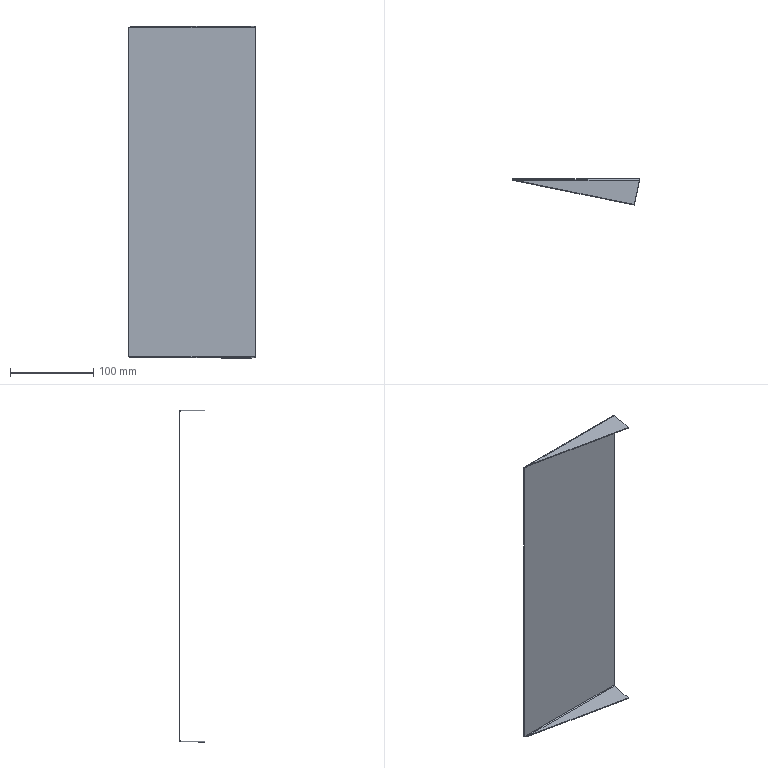Part | 1 solid | 20 faces | box 152.5 x 31 x 399 mm | volume 65219 mm3 | plane 12 | spline 4 | cylinder 4 | commonest cylinder face diameters 2 x2 4 x2
STEP:
#1=CARTESIAN_POINT('',(0.,-1.,-197.5));
#2=VERTEX_POINT('',#1);
#3=CARTESIAN_POINT('',(-152.5,-1.,-197.5));
#4=VERTEX_POINT('',#3);
#5=CARTESIAN_POINT('',(0.,-1.,-197.5));
#6=DIRECTION('',(-1.,0.,0.));
#7=VECTOR('',#6,1000.);
#8=LINE('',#5,#7);
#9=EDGE_CURVE('',#2,#4,#8,.T.);
#10=ORIENTED_EDGE('',*,*,#9,.F.);
#11=CARTESIAN_POINT('',(0.,-1.,197.5));
#12=VERTEX_POINT('',#11);
#13=CARTESIAN_POINT('',(0.,-1.,199.5));
#14=DIRECTION('',(0.,0.,-1.));
#15=VECTOR('',#14,1000.);
#16=LINE('',#13,#15);
#17=EDGE_CURVE('',#12,#2,#16,.T.);
#18=ORIENTED_EDGE('',*,*,#17,.F.);
#19=CARTESIAN_POINT('',(-152.5,-1.,197.5));
#20=VERTEX_POINT('',#19);
#21=CARTESIAN_POINT('',(-152.5,-1.,197.5));
#22=DIRECTION('',(1.,0.,0.));
#23=VECTOR('',#22,1000.);
#24=LINE('',#21,#23);
#25=EDGE_CURVE('',#20,#12,#24,.T.);
#26=ORIENTED_EDGE('',*,*,#25,.F.);
#27=CARTESIAN_POINT('',(-152.5,-1.,199.5));
#28=DIRECTION('',(0.,0.,-1.));
#29=VECTOR('',#28,1000.);
#30=LINE('',#27,#29);
#31=EDGE_CURVE('',#20,#4,#30,.T.);
#32=ORIENTED_EDGE('',*,*,#31,.T.);
#33=EDGE_LOOP('',(#10,#18,#26,#32));
#34=FACE_OUTER_BOUND('',#33,.T.);
#35=CARTESIAN_POINT('',(-152.5,-1.,199.5));
#36=DIRECTION('',(0.,1.,0.));
#37=DIRECTION('',(0.,0.,1.));
#38=AXIS2_PLACEMENT_3D('',#35,#36,#37);
#39=PLANE('',#38);
#40=ADVANCED_FACE('',(#34),#39,.F.);
#41=CARTESIAN_POINT('',(0.,0.,197.5));
#42=VERTEX_POINT('',#41);
#43=CARTESIAN_POINT('',(0.,0.,-197.5));
#44=VERTEX_POINT('',#43);
#45=CARTESIAN_POINT('',(0.,0.,199.5));
#46=DIRECTION('',(0.,0.,-1.));
#47=VECTOR('',#46,1000.);
#48=LINE('',#45,#47);
#49=EDGE_CURVE('',#42,#44,#48,.T.);
#50=ORIENTED_EDGE('',*,*,#49,.T.);
#51=CARTESIAN_POINT('',(-152.5,0.,-197.5));
#52=VERTEX_POINT('',#51);
#53=CARTESIAN_POINT('',(0.,0.,-197.5));
#54=DIRECTION('',(-1.,0.,0.));
#55=VECTOR('',#54,1000.);
#56=LINE('',#53,#55);
#57=EDGE_CURVE('',#44,#52,#56,.T.);
#58=ORIENTED_EDGE('',*,*,#57,.T.);
#59=CARTESIAN_POINT('',(-152.5,0.,197.5));
#60=VERTEX_POINT('',#59);
#61=CARTESIAN_POINT('',(-152.5,0.,199.5));
#62=DIRECTION('',(0.,0.,-1.));
#63=VECTOR('',#62,1000.);
#64=LINE('',#61,#63);
#65=EDGE_CURVE('',#60,#52,#64,.T.);
#66=ORIENTED_EDGE('',*,*,#65,.F.);
#67=CARTESIAN_POINT('',(-152.5,0.,197.5));
#68=DIRECTION('',(1.,0.,0.));
#69=VECTOR('',#68,1000.);
#70=LINE('',#67,#69);
#71=EDGE_CURVE('',#60,#42,#70,.T.);
#72=ORIENTED_EDGE('',*,*,#71,.T.);
#73=EDGE_LOOP('',(#50,#58,#66,#72));
#74=FACE_OUTER_BOUND('',#73,.T.);
#75=CARTESIAN_POINT('',(-152.5,0.,199.5));
#76=DIRECTION('',(0.,1.,0.));
#77=DIRECTION('',(0.,0.,1.));
#78=AXIS2_PLACEMENT_3D('',#75,#76,#77);
#79=PLANE('',#78);
#80=ADVANCED_FACE('',(#74),#79,.T.);
#81=ORIENTED_EDGE('',*,*,#17,.T.);
#82=CARTESIAN_POINT('',(0.,-1.,-197.5));
#83=DIRECTION('',(0.,1.,0.));
#84=VECTOR('',#83,1000.);
#85=LINE('',#82,#84);
#86=EDGE_CURVE('',#2,#44,#85,.T.);
#87=ORIENTED_EDGE('',*,*,#86,.T.);
#88=ORIENTED_EDGE('',*,*,#49,.F.);
#89=CARTESIAN_POINT('',(0.,-1.,197.5));
#90=DIRECTION('',(0.,1.,0.));
#91=VECTOR('',#90,1000.);
#92=LINE('',#89,#91);
#93=EDGE_CURVE('',#12,#42,#92,.T.);
#94=ORIENTED_EDGE('',*,*,#93,.F.);
#95=EDGE_LOOP('',(#81,#87,#88,#94));
#96=FACE_OUTER_BOUND('',#95,.T.);
#97=CARTESIAN_POINT('',(0.,0.,199.5));
#98=DIRECTION('',(1.,0.,0.));
#99=DIRECTION('',(0.,0.,-1.));
#100=AXIS2_PLACEMENT_3D('',#97,#98,#99);
#101=PLANE('',#100);
#102=ADVANCED_FACE('',(#96),#101,.T.);
#103=CARTESIAN_POINT('',(-152.5,-1.,-197.5));
#104=DIRECTION('',(0.,1.,0.));
#105=VECTOR('',#104,1000.);
#106=LINE('',#103,#105);
#107=EDGE_CURVE('',#4,#52,#106,.T.);
#108=ORIENTED_EDGE('',*,*,#107,.F.);
#109=ORIENTED_EDGE('',*,*,#31,.F.);
#110=CARTESIAN_POINT('',(-152.5,-1.,197.5));
#111=DIRECTION('',(0.,1.,0.));
#112=VECTOR('',#111,1000.);
#113=LINE('',#110,#112);
#114=EDGE_CURVE('',#20,#60,#113,.T.);
#115=ORIENTED_EDGE('',*,*,#114,.T.);
#116=ORIENTED_EDGE('',*,*,#65,.T.);
#117=EDGE_LOOP('',(#108,#109,#115,#116));
#118=FACE_OUTER_BOUND('',#117,.T.);
#119=CARTESIAN_POINT('',(-152.5,-1.,199.5));
#120=DIRECTION('',(-1.,0.,0.));
#121=DIRECTION('',(0.,0.,1.));
#122=AXIS2_PLACEMENT_3D('',#119,#120,#121);
#123=PLANE('',#122);
#124=ADVANCED_FACE('',(#118),#123,.T.);
#125=CARTESIAN_POINT('',(-0.205,-2.,198.5));
#126=VERTEX_POINT('',#125);
#127=CARTESIAN_POINT('',(-0.205,-2.,199.5));
#128=VERTEX_POINT('',#127);
#129=CARTESIAN_POINT('',(-0.205,-2.,199.5));
#130=DIRECTION('',(0.,0.,1.));
#131=VECTOR('',#130,1000.);
#132=LINE('',#129,#131);
#133=EDGE_CURVE('',#126,#128,#132,.T.);
#134=ORIENTED_EDGE('',*,*,#133,.F.);
#135=CARTESIAN_POINT('',(0.,-1.,197.5));
#136=CARTESIAN_POINT('',(-0.03416,-1.,197.762));
#137=CARTESIAN_POINT('',(-0.06833,-1.108,198.022));
#138=CARTESIAN_POINT('',(-0.1367,-1.478,198.392));
#139=CARTESIAN_POINT('',(-0.1708,-1.738,198.5));
#140=CARTESIAN_POINT('',(-0.205,-2.,198.5));
#141=B_SPLINE_CURVE_WITH_KNOTS('',3,(#135,#136,#137,#138,#139,#140),.UNSPECIFIED.,.F.,.F.,(4,2,4),(0.,0.5,1.),.UNSPECIFIED.);
#142=EDGE_CURVE('',#12,#126,#141,.T.);
#143=ORIENTED_EDGE('',*,*,#142,.F.);
#144=ORIENTED_EDGE('',*,*,#93,.T.);
#145=CARTESIAN_POINT('',(0.,0.,197.5));
#146=CARTESIAN_POINT('',(-0.01708,0.,197.762));
#147=CARTESIAN_POINT('',(-0.03416,-0.05205,198.023));
#148=CARTESIAN_POINT('',(-0.06833,-0.2524,198.507));
#149=CARTESIAN_POINT('',(-0.08541,-0.4007,198.729));
#150=CARTESIAN_POINT('',(-0.1196,-0.7709,199.099));
#151=CARTESIAN_POINT('',(-0.1367,-0.9928,199.248));
#152=CARTESIAN_POINT('',(-0.1708,-1.477,199.448));
#153=CARTESIAN_POINT('',(-0.1879,-1.738,199.5));
#154=CARTESIAN_POINT('',(-0.205,-2.,199.5));
#155=B_SPLINE_CURVE_WITH_KNOTS('',3,(#145,#146,#147,#148,#149,#150,#151,#152,#153,#154),.UNSPECIFIED.,.F.,.F.,(4,2,2,2,4),(0.,0.25,0.5,0.75,1.),.UNSPECIFIED.);
#156=EDGE_CURVE('',#42,#128,#155,.T.);
#157=ORIENTED_EDGE('',*,*,#156,.T.);
#158=EDGE_LOOP('',(#134,#143,#144,#157));
#159=FACE_OUTER_BOUND('',#158,.T.);
#160=CARTESIAN_POINT('',(0.,0.01,197.5));
#161=CARTESIAN_POINT('',(-0.01709,0.01,197.763));
#162=CARTESIAN_POINT('',(-0.03416,-0.04231,198.026));
#163=CARTESIAN_POINT('',(-0.06833,-0.2437,198.512));
#164=CARTESIAN_POINT('',(-0.08541,-0.3927,198.735));
#165=CARTESIAN_POINT('',(-0.1196,-0.7648,199.107));
#166=CARTESIAN_POINT('',(-0.1367,-0.9877,199.256));
#167=CARTESIAN_POINT('',(-0.1708,-1.474,199.458));
#168=CARTESIAN_POINT('',(-0.1879,-1.737,199.51));
#169=CARTESIAN_POINT('',(-0.205,-2.,199.51));
#170=CARTESIAN_POINT('',(0.,0.,197.5));
#171=CARTESIAN_POINT('',(-0.01709,0.,197.762));
#172=CARTESIAN_POINT('',(-0.03416,-0.05205,198.023));
#173=CARTESIAN_POINT('',(-0.06833,-0.2524,198.507));
#174=CARTESIAN_POINT('',(-0.08541,-0.4007,198.729));
#175=CARTESIAN_POINT('',(-0.1196,-0.7709,199.099));
#176=CARTESIAN_POINT('',(-0.1367,-0.9928,199.248));
#177=CARTESIAN_POINT('',(-0.1708,-1.477,199.448));
#178=CARTESIAN_POINT('',(-0.1879,-1.738,199.5));
#179=CARTESIAN_POINT('',(-0.205,-2.,199.5));
#180=CARTESIAN_POINT('',(0.,-1.,197.5));
#181=CARTESIAN_POINT('',(-0.01709,-1.,197.631));
#182=CARTESIAN_POINT('',(-0.03416,-1.026,197.762));
#183=CARTESIAN_POINT('',(-0.06833,-1.126,198.004));
#184=CARTESIAN_POINT('',(-0.08541,-1.2,198.115));
#185=CARTESIAN_POINT('',(-0.1196,-1.385,198.3));
#186=CARTESIAN_POINT('',(-0.1367,-1.496,198.374));
#187=CARTESIAN_POINT('',(-0.1708,-1.738,198.474));
#188=CARTESIAN_POINT('',(-0.1879,-1.869,198.5));
#189=CARTESIAN_POINT('',(-0.205,-2.,198.5));
#190=CARTESIAN_POINT('',(0.,-1.01,197.5));
#191=CARTESIAN_POINT('',(-0.01709,-1.01,197.63));
#192=CARTESIAN_POINT('',(-0.03416,-1.036,197.759));
#193=CARTESIAN_POINT('',(-0.06833,-1.135,197.999));
#194=CARTESIAN_POINT('',(-0.08541,-1.208,198.108));
#195=CARTESIAN_POINT('',(-0.1196,-1.392,198.292));
#196=CARTESIAN_POINT('',(-0.1367,-1.501,198.365));
#197=CARTESIAN_POINT('',(-0.1708,-1.741,198.464));
#198=CARTESIAN_POINT('',(-0.1879,-1.87,198.49));
#199=CARTESIAN_POINT('',(-0.205,-2.,198.49));
#200=B_SPLINE_SURFACE_WITH_KNOTS('',1,3,((#160,#161,#162,#163,#164,#165,#166,#167,#168,#169),(#170,#171,#172,#173,#174,#175,#176,#177,#178,#179),(#180,#181,#182,#183,#184,#185,#186,#187,#188,#189),(#190,#191,#192,#193,#194,#195,#196,#197,#198,#199)),.UNSPECIFIED.,.F.,.F.,.F.,(2,1,1,2),(4,2,2,2,4),(-0.01,0.,1.,1.01),(0.,0.25,0.5,0.75,1.),.UNSPECIFIED.);
#201=ADVANCED_FACE('',(#159),#200,.F.);
#202=CARTESIAN_POINT('',(-147.622,-2.,198.5));
#203=VERTEX_POINT('',#202);
#204=CARTESIAN_POINT('',(-147.622,-2.,198.5));
#205=CARTESIAN_POINT('',(-148.029,-1.869,198.5));
#206=CARTESIAN_POINT('',(-148.434,-1.738,198.474));
#207=CARTESIAN_POINT('',(-149.246,-1.497,198.374));
#208=CARTESIAN_POINT('',(-149.653,-1.386,198.3));
#209=CARTESIAN_POINT('',(-150.466,-1.201,198.115));
#210=CARTESIAN_POINT('',(-150.873,-1.126,198.004));
#211=CARTESIAN_POINT('',(-151.687,-1.026,197.762));
#212=CARTESIAN_POINT('',(-152.093,-1.,197.631));
#213=CARTESIAN_POINT('',(-152.5,-1.,197.5));
#214=B_SPLINE_CURVE_WITH_KNOTS('',3,(#204,#205,#206,#207,#208,#209,#210,#211,#212,#213),.UNSPECIFIED.,.F.,.F.,(4,2,2,2,4),(0.,0.001278,0.002557,0.003835,0.005114),.UNSPECIFIED.);
#215=EDGE_CURVE('',#203,#20,#214,.T.);
#216=ORIENTED_EDGE('',*,*,#215,.F.);
#217=CARTESIAN_POINT('',(-147.622,-2.,199.5));
#218=VERTEX_POINT('',#217);
#219=CARTESIAN_POINT('',(-147.622,-2.,198.5));
#220=DIRECTION('',(0.,0.,1.));
#221=VECTOR('',#220,1000.);
#222=LINE('',#219,#221);
#223=EDGE_CURVE('',#203,#218,#222,.T.);
#224=ORIENTED_EDGE('',*,*,#223,.T.);
#225=CARTESIAN_POINT('',(-147.622,-2.,199.5));
#226=CARTESIAN_POINT('',(-148.031,-1.736,199.5));
#227=CARTESIAN_POINT('',(-148.434,-1.477,199.448));
#228=CARTESIAN_POINT('',(-149.245,-0.9944,199.248));
#229=CARTESIAN_POINT('',(-149.655,-0.7707,199.099));
#230=CARTESIAN_POINT('',(-150.262,-0.4941,198.823));
#231=CARTESIAN_POINT('',(-150.464,-0.411,198.722));
#232=CARTESIAN_POINT('',(-150.87,-0.2655,198.504));
#233=CARTESIAN_POINT('',(-151.075,-0.2028,198.387));
#234=CARTESIAN_POINT('',(-151.687,-0.05199,198.024));
#235=CARTESIAN_POINT('',(-152.091,0.,197.764));
#236=CARTESIAN_POINT('',(-152.5,0.,197.5));
#237=B_SPLINE_CURVE_WITH_KNOTS('',3,(#225,#226,#227,#228,#229,#230,#231,#232,#233,#234,#235,#236),.UNSPECIFIED.,.F.,.F.,(4,2,2,2,2,4),(0.,0.001444,0.002888,0.003611,0.004333,0.005777),.UNSPECIFIED.);
#238=EDGE_CURVE('',#218,#60,#237,.T.);
#239=ORIENTED_EDGE('',*,*,#238,.T.);
#240=ORIENTED_EDGE('',*,*,#114,.F.);
#241=EDGE_LOOP('',(#216,#224,#239,#240));
#242=FACE_OUTER_BOUND('',#241,.T.);
#243=CARTESIAN_POINT('',(-147.622,-2.,199.51));
#244=CARTESIAN_POINT('',(-148.028,-1.737,199.51));
#245=CARTESIAN_POINT('',(-148.435,-1.474,199.458));
#246=CARTESIAN_POINT('',(-149.248,-0.9877,199.256));
#247=CARTESIAN_POINT('',(-149.654,-0.7648,199.107));
#248=CARTESIAN_POINT('',(-150.467,-0.3927,198.735));
#249=CARTESIAN_POINT('',(-150.874,-0.2437,198.512));
#250=CARTESIAN_POINT('',(-151.687,-0.04231,198.026));
#251=CARTESIAN_POINT('',(-152.093,0.01,197.763));
#252=CARTESIAN_POINT('',(-152.5,0.01,197.5));
#253=CARTESIAN_POINT('',(-147.622,-2.,199.5));
#254=CARTESIAN_POINT('',(-148.028,-1.738,199.5));
#255=CARTESIAN_POINT('',(-148.435,-1.477,199.448));
#256=CARTESIAN_POINT('',(-149.248,-0.9928,199.248));
#257=CARTESIAN_POINT('',(-149.654,-0.7709,199.099));
#258=CARTESIAN_POINT('',(-150.467,-0.4007,198.729));
#259=CARTESIAN_POINT('',(-150.874,-0.2524,198.507));
#260=CARTESIAN_POINT('',(-151.687,-0.05205,198.023));
#261=CARTESIAN_POINT('',(-152.093,0.,197.762));
#262=CARTESIAN_POINT('',(-152.5,0.,197.5));
#263=CARTESIAN_POINT('',(-147.622,-2.,198.5));
#264=CARTESIAN_POINT('',(-148.028,-1.869,198.5));
#265=CARTESIAN_POINT('',(-148.435,-1.738,198.474));
#266=CARTESIAN_POINT('',(-149.248,-1.496,198.374));
#267=CARTESIAN_POINT('',(-149.654,-1.385,198.3));
#268=CARTESIAN_POINT('',(-150.467,-1.2,198.115));
#269=CARTESIAN_POINT('',(-150.874,-1.126,198.004));
#270=CARTESIAN_POINT('',(-151.687,-1.026,197.762));
#271=CARTESIAN_POINT('',(-152.093,-1.,197.631));
#272=CARTESIAN_POINT('',(-152.5,-1.,197.5));
#273=CARTESIAN_POINT('',(-147.622,-2.,198.49));
#274=CARTESIAN_POINT('',(-148.028,-1.87,198.49));
#275=CARTESIAN_POINT('',(-148.435,-1.741,198.464));
#276=CARTESIAN_POINT('',(-149.248,-1.501,198.365));
#277=CARTESIAN_POINT('',(-149.654,-1.392,198.292));
#278=CARTESIAN_POINT('',(-150.467,-1.208,198.108));
#279=CARTESIAN_POINT('',(-150.874,-1.135,197.999));
#280=CARTESIAN_POINT('',(-151.687,-1.036,197.759));
#281=CARTESIAN_POINT('',(-152.093,-1.01,197.63));
#282=CARTESIAN_POINT('',(-152.5,-1.01,197.5));
#283=B_SPLINE_SURFACE_WITH_KNOTS('',1,3,((#243,#244,#245,#246,#247,#248,#249,#250,#251,#252),(#253,#254,#255,#256,#257,#258,#259,#260,#261,#262),(#263,#264,#265,#266,#267,#268,#269,#270,#271,#272),(#273,#274,#275,#276,#277,#278,#279,#280,#281,#282)),.UNSPECIFIED.,.F.,.F.,.F.,(2,1,1,2),(4,2,2,2,4),(-0.01,0.,1.,1.01),(0.,0.25,0.5,0.75,1.),.UNSPECIFIED.);
#284=ADVANCED_FACE('',(#242),#283,.F.);
#285=ORIENTED_EDGE('',*,*,#71,.F.);
#286=ORIENTED_EDGE('',*,*,#238,.F.);
#287=CARTESIAN_POINT('',(-0.205,-2.,199.5));
#288=DIRECTION('',(1.,0.,0.));
#289=VECTOR('',#288,1000.);
#290=LINE('',#287,#289);
#291=EDGE_CURVE('',#218,#128,#290,.T.);
#292=ORIENTED_EDGE('',*,*,#291,.T.);
#293=ORIENTED_EDGE('',*,*,#156,.F.);
#294=EDGE_LOOP('',(#285,#286,#292,#293));
#295=FACE_OUTER_BOUND('',#294,.T.);
#296=CARTESIAN_POINT('',(-152.5,-2.,197.5));
#297=DIRECTION('',(-1.,0.,0.));
#298=DIRECTION('',(0.,0.,1.));
#299=AXIS2_PLACEMENT_3D('',#296,#297,#298);
#300=CYLINDRICAL_SURFACE('',#299,2.);
#301=ADVANCED_FACE('',(#295),#300,.T.);
#302=ORIENTED_EDGE('',*,*,#25,.T.);
#303=ORIENTED_EDGE('',*,*,#142,.T.);
#304=CARTESIAN_POINT('',(-0.205,-2.,198.5));
#305=DIRECTION('',(-1.,0.,0.));
#306=VECTOR('',#305,1000.);
#307=LINE('',#304,#306);
#308=EDGE_CURVE('',#126,#203,#307,.T.);
#309=ORIENTED_EDGE('',*,*,#308,.T.);
#310=ORIENTED_EDGE('',*,*,#215,.T.);
#311=EDGE_LOOP('',(#302,#303,#309,#310));
#312=FACE_OUTER_BOUND('',#311,.T.);
#313=CARTESIAN_POINT('',(-152.5,-2.,197.5));
#314=DIRECTION('',(-1.,0.,0.));
#315=DIRECTION('',(0.,0.,1.));
#316=AXIS2_PLACEMENT_3D('',#313,#314,#315);
#317=CYLINDRICAL_SURFACE('',#316,1.);
#318=ADVANCED_FACE('',(#312),#317,.F.);
#319=CARTESIAN_POINT('',(-6.15,-31.,199.5));
#320=VERTEX_POINT('',#319);
#321=CARTESIAN_POINT('',(-152.5,-1.,199.5));
#322=DIRECTION('',(-0.9796,0.2008,0.));
#323=VECTOR('',#322,1000.);
#324=LINE('',#321,#323);
#325=EDGE_CURVE('',#320,#218,#324,.T.);
#326=ORIENTED_EDGE('',*,*,#325,.T.);
#327=ORIENTED_EDGE('',*,*,#223,.F.);
#328=CARTESIAN_POINT('',(-6.15,-31.,198.5));
#329=VERTEX_POINT('',#328);
#330=CARTESIAN_POINT('',(-6.346,-30.96,198.5));
#331=DIRECTION('',(-0.9796,0.2008,0.));
#332=VECTOR('',#331,1000.);
#333=LINE('',#330,#332);
#334=EDGE_CURVE('',#329,#203,#333,.T.);
#335=ORIENTED_EDGE('',*,*,#334,.F.);
#336=CARTESIAN_POINT('',(-6.15,-31.,199.5));
#337=DIRECTION('',(0.,0.,-1.));
#338=VECTOR('',#337,1000.);
#339=LINE('',#336,#338);
#340=EDGE_CURVE('',#320,#329,#339,.T.);
#341=ORIENTED_EDGE('',*,*,#340,.F.);
#342=EDGE_LOOP('',(#326,#327,#335,#341));
#343=FACE_OUTER_BOUND('',#342,.T.);
#344=CARTESIAN_POINT('',(-152.5,-1.,199.5));
#345=DIRECTION('',(-0.2008,-0.9796,0.));
#346=DIRECTION('',(0.9796,-0.2008,0.));
#347=AXIS2_PLACEMENT_3D('',#344,#345,#346);
#348=PLANE('',#347);
#349=ADVANCED_FACE('',(#343),#348,.T.);
#350=CARTESIAN_POINT('',(0.1967,-0.04033,198.5));
#351=DIRECTION('',(-0.2008,-0.9796,0.));
#352=VECTOR('',#351,1000.);
#353=LINE('',#350,#352);
#354=EDGE_CURVE('',#126,#329,#353,.T.);
#355=ORIENTED_EDGE('',*,*,#354,.F.);
#356=ORIENTED_EDGE('',*,*,#133,.T.);
#357=CARTESIAN_POINT('',(-6.15,-31.,199.5));
#358=DIRECTION('',(-0.2008,-0.9796,0.));
#359=VECTOR('',#358,1000.);
#360=LINE('',#357,#359);
#361=EDGE_CURVE('',#128,#320,#360,.T.);
#362=ORIENTED_EDGE('',*,*,#361,.T.);
#363=ORIENTED_EDGE('',*,*,#340,.T.);
#364=EDGE_LOOP('',(#355,#356,#362,#363));
#365=FACE_OUTER_BOUND('',#364,.T.);
#366=CARTESIAN_POINT('',(-6.15,-31.,199.5));
#367=DIRECTION('',(0.9796,-0.2008,0.));
#368=DIRECTION('',(0.2008,0.9796,0.));
#369=AXIS2_PLACEMENT_3D('',#366,#367,#368);
#370=PLANE('',#369);
#371=ADVANCED_FACE('',(#365),#370,.T.);
#372=ORIENTED_EDGE('',*,*,#291,.F.);
#373=ORIENTED_EDGE('',*,*,#325,.F.);
#374=ORIENTED_EDGE('',*,*,#361,.F.);
#375=EDGE_LOOP('',(#372,#373,#374));
#376=FACE_OUTER_BOUND('',#375,.T.);
#377=CARTESIAN_POINT('',(0.,0.,199.5));
#378=DIRECTION('',(0.,0.,-1.));
#379=DIRECTION('',(0.,1.,0.));
#380=AXIS2_PLACEMENT_3D('',#377,#378,#379);
#381=PLANE('',#380);
#382=ADVANCED_FACE('',(#376),#381,.F.);
#383=ORIENTED_EDGE('',*,*,#334,.T.);
#384=ORIENTED_EDGE('',*,*,#308,.F.);
#385=ORIENTED_EDGE('',*,*,#354,.T.);
#386=EDGE_LOOP('',(#383,#384,#385));
#387=FACE_OUTER_BOUND('',#386,.T.);
#388=CARTESIAN_POINT('',(0.,0.,198.5));
#389=DIRECTION('',(0.,0.,-1.));
#390=DIRECTION('',(0.,1.,0.));
#391=AXIS2_PLACEMENT_3D('',#388,#389,#390);
#392=PLANE('',#391);
#393=ADVANCED_FACE('',(#387),#392,.T.);
#394=CARTESIAN_POINT('',(-147.622,-2.,-198.5));
#395=VERTEX_POINT('',#394);
#396=CARTESIAN_POINT('',(-147.622,-2.,-199.5));
#397=VERTEX_POINT('',#396);
#398=CARTESIAN_POINT('',(-147.622,-2.,-199.5));
#399=DIRECTION('',(0.,0.,-1.));
#400=VECTOR('',#399,1000.);
#401=LINE('',#398,#400);
#402=EDGE_CURVE('',#395,#397,#401,.T.);
#403=ORIENTED_EDGE('',*,*,#402,.F.);
#404=CARTESIAN_POINT('',(-152.5,-1.,-197.5));
#405=CARTESIAN_POINT('',(-152.093,-1.,-197.631));
#406=CARTESIAN_POINT('',(-151.687,-1.026,-197.762));
#407=CARTESIAN_POINT('',(-150.876,-1.126,-198.003));
#408=CARTESIAN_POINT('',(-150.468,-1.2,-198.114));
#409=CARTESIAN_POINT('',(-149.655,-1.385,-198.299));
#410=CARTESIAN_POINT('',(-149.248,-1.496,-198.374));
#411=CARTESIAN_POINT('',(-148.435,-1.738,-198.474));
#412=CARTESIAN_POINT('',(-148.029,-1.869,-198.5));
#413=CARTESIAN_POINT('',(-147.622,-2.,-198.5));
#414=B_SPLINE_CURVE_WITH_KNOTS('',3,(#404,#405,#406,#407,#408,#409,#410,#411,#412,#413),.UNSPECIFIED.,.F.,.F.,(4,2,2,2,4),(0.,0.001278,0.002557,0.003835,0.005114),.UNSPECIFIED.);
#415=EDGE_CURVE('',#4,#395,#414,.T.);
#416=ORIENTED_EDGE('',*,*,#415,.F.);
#417=ORIENTED_EDGE('',*,*,#107,.T.);
#418=CARTESIAN_POINT('',(-152.5,0.,-197.5));
#419=CARTESIAN_POINT('',(-152.091,0.,-197.764));
#420=CARTESIAN_POINT('',(-151.688,-0.05198,-198.023));
#421=CARTESIAN_POINT('',(-150.877,-0.2516,-198.506));
#422=CARTESIAN_POINT('',(-150.467,-0.401,-198.729));
#423=CARTESIAN_POINT('',(-149.859,-0.6774,-199.006));
#424=CARTESIAN_POINT('',(-149.657,-0.7785,-199.089));
#425=CARTESIAN_POINT('',(-149.251,-0.9958,-199.235));
#426=CARTESIAN_POINT('',(-149.046,-1.113,-199.297));
#427=CARTESIAN_POINT('',(-148.435,-1.476,-199.448));
#428=CARTESIAN_POINT('',(-148.031,-1.736,-199.5));
#429=CARTESIAN_POINT('',(-147.622,-2.,-199.5));
#430=B_SPLINE_CURVE_WITH_KNOTS('',3,(#418,#419,#420,#421,#422,#423,#424,#425,#426,#427,#428,#429),.UNSPECIFIED.,.F.,.F.,(4,2,2,2,2,4),(0.,0.001444,0.002888,0.003611,0.004333,0.005777),.UNSPECIFIED.);
#431=EDGE_CURVE('',#52,#397,#430,.T.);
#432=ORIENTED_EDGE('',*,*,#431,.T.);
#433=EDGE_LOOP('',(#403,#416,#417,#432));
#434=FACE_OUTER_BOUND('',#433,.T.);
#435=CARTESIAN_POINT('',(-152.5,0.01,-197.5));
#436=CARTESIAN_POINT('',(-152.093,0.01,-197.763));
#437=CARTESIAN_POINT('',(-151.687,-0.04231,-198.026));
#438=CARTESIAN_POINT('',(-150.874,-0.2437,-198.512));
#439=CARTESIAN_POINT('',(-150.467,-0.3927,-198.735));
#440=CARTESIAN_POINT('',(-149.654,-0.7648,-199.107));
#441=CARTESIAN_POINT('',(-149.248,-0.9877,-199.256));
#442=CARTESIAN_POINT('',(-148.435,-1.474,-199.458));
#443=CARTESIAN_POINT('',(-148.028,-1.737,-199.51));
#444=CARTESIAN_POINT('',(-147.622,-2.,-199.51));
#445=CARTESIAN_POINT('',(-152.5,0.,-197.5));
#446=CARTESIAN_POINT('',(-152.093,0.,-197.762));
#447=CARTESIAN_POINT('',(-151.687,-0.05205,-198.023));
#448=CARTESIAN_POINT('',(-150.874,-0.2524,-198.507));
#449=CARTESIAN_POINT('',(-150.467,-0.4007,-198.729));
#450=CARTESIAN_POINT('',(-149.654,-0.7709,-199.099));
#451=CARTESIAN_POINT('',(-149.248,-0.9928,-199.248));
#452=CARTESIAN_POINT('',(-148.435,-1.477,-199.448));
#453=CARTESIAN_POINT('',(-148.028,-1.738,-199.5));
#454=CARTESIAN_POINT('',(-147.622,-2.,-199.5));
#455=CARTESIAN_POINT('',(-152.5,-1.,-197.5));
#456=CARTESIAN_POINT('',(-152.093,-1.,-197.631));
#457=CARTESIAN_POINT('',(-151.687,-1.026,-197.762));
#458=CARTESIAN_POINT('',(-150.874,-1.126,-198.004));
#459=CARTESIAN_POINT('',(-150.467,-1.2,-198.115));
#460=CARTESIAN_POINT('',(-149.654,-1.385,-198.3));
#461=CARTESIAN_POINT('',(-149.248,-1.496,-198.374));
#462=CARTESIAN_POINT('',(-148.435,-1.738,-198.474));
#463=CARTESIAN_POINT('',(-148.028,-1.869,-198.5));
#464=CARTESIAN_POINT('',(-147.622,-2.,-198.5));
#465=CARTESIAN_POINT('',(-152.5,-1.01,-197.5));
#466=CARTESIAN_POINT('',(-152.093,-1.01,-197.63));
#467=CARTESIAN_POINT('',(-151.687,-1.036,-197.759));
#468=CARTESIAN_POINT('',(-150.874,-1.135,-197.999));
#469=CARTESIAN_POINT('',(-150.467,-1.208,-198.108));
#470=CARTESIAN_POINT('',(-149.654,-1.392,-198.292));
#471=CARTESIAN_POINT('',(-149.248,-1.501,-198.365));
#472=CARTESIAN_POINT('',(-148.435,-1.741,-198.464));
#473=CARTESIAN_POINT('',(-148.028,-1.87,-198.49));
#474=CARTESIAN_POINT('',(-147.622,-2.,-198.49));
#475=B_SPLINE_SURFACE_WITH_KNOTS('',1,3,((#435,#436,#437,#438,#439,#440,#441,#442,#443,#444),(#445,#446,#447,#448,#449,#450,#451,#452,#453,#454),(#455,#456,#457,#458,#459,#460,#461,#462,#463,#464),(#465,#466,#467,#468,#469,#470,#471,#472,#473,#474)),.UNSPECIFIED.,.F.,.F.,.F.,(2,1,1,2),(4,2,2,2,4),(-0.01,0.,1.,1.01),(0.,0.25,0.5,0.75,1.),.UNSPECIFIED.);
#476=ADVANCED_FACE('',(#434),#475,.F.);
#477=CARTESIAN_POINT('',(-0.205,-2.,-198.5));
#478=VERTEX_POINT('',#477);
#479=CARTESIAN_POINT('',(-0.205,-2.,-198.5));
#480=CARTESIAN_POINT('',(-0.1708,-1.738,-198.5));
#481=CARTESIAN_POINT('',(-0.1367,-1.478,-198.392));
#482=CARTESIAN_POINT('',(-0.06833,-1.108,-198.022));
#483=CARTESIAN_POINT('',(-0.03416,-1.,-197.762));
#484=CARTESIAN_POINT('',(0.,-1.,-197.5));
#485=B_SPLINE_CURVE_WITH_KNOTS('',3,(#479,#480,#481,#482,#483,#484),.UNSPECIFIED.,.F.,.F.,(4,2,4),(0.,0.5,1.),.UNSPECIFIED.);
#486=EDGE_CURVE('',#478,#2,#485,.T.);
#487=ORIENTED_EDGE('',*,*,#486,.F.);
#488=CARTESIAN_POINT('',(-0.205,-2.,-199.5));
#489=VERTEX_POINT('',#488);
#490=CARTESIAN_POINT('',(-0.205,-2.,-198.5));
#491=DIRECTION('',(0.,0.,-1.));
#492=VECTOR('',#491,1000.);
#493=LINE('',#490,#492);
#494=EDGE_CURVE('',#478,#489,#493,.T.);
#495=ORIENTED_EDGE('',*,*,#494,.T.);
#496=CARTESIAN_POINT('',(-0.205,-2.,-199.5));
#497=CARTESIAN_POINT('',(-0.1879,-1.738,-199.5));
#498=CARTESIAN_POINT('',(-0.1708,-1.477,-199.448));
#499=CARTESIAN_POINT('',(-0.1367,-0.9928,-199.248));
#500=CARTESIAN_POINT('',(-0.1196,-0.7709,-199.099));
#501=CARTESIAN_POINT('',(-0.08541,-0.4007,-198.729));
#502=CARTESIAN_POINT('',(-0.06833,-0.2524,-198.507));
#503=CARTESIAN_POINT('',(-0.03416,-0.05205,-198.023));
#504=CARTESIAN_POINT('',(-0.01708,0.,-197.762));
#505=CARTESIAN_POINT('',(0.,0.,-197.5));
#506=B_SPLINE_CURVE_WITH_KNOTS('',3,(#496,#497,#498,#499,#500,#501,#502,#503,#504,#505),.UNSPECIFIED.,.F.,.F.,(4,2,2,2,4),(0.,0.25,0.5,0.75,1.),.UNSPECIFIED.);
#507=EDGE_CURVE('',#489,#44,#506,.T.);
#508=ORIENTED_EDGE('',*,*,#507,.T.);
#509=ORIENTED_EDGE('',*,*,#86,.F.);
#510=EDGE_LOOP('',(#487,#495,#508,#509));
#511=FACE_OUTER_BOUND('',#510,.T.);
#512=CARTESIAN_POINT('',(-0.205,-2.,-199.51));
#513=CARTESIAN_POINT('',(-0.1879,-1.737,-199.51));
#514=CARTESIAN_POINT('',(-0.1708,-1.474,-199.458));
#515=CARTESIAN_POINT('',(-0.1367,-0.9877,-199.256));
#516=CARTESIAN_POINT('',(-0.1196,-0.7648,-199.107));
#517=CARTESIAN_POINT('',(-0.08541,-0.3927,-198.735));
#518=CARTESIAN_POINT('',(-0.06833,-0.2437,-198.512));
#519=CARTESIAN_POINT('',(-0.03416,-0.04231,-198.026));
#520=CARTESIAN_POINT('',(-0.01709,0.01,-197.763));
#521=CARTESIAN_POINT('',(0.,0.01,-197.5));
#522=CARTESIAN_POINT('',(-0.205,-2.,-199.5));
#523=CARTESIAN_POINT('',(-0.1879,-1.738,-199.5));
#524=CARTESIAN_POINT('',(-0.1708,-1.477,-199.448));
#525=CARTESIAN_POINT('',(-0.1367,-0.9928,-199.248));
#526=CARTESIAN_POINT('',(-0.1196,-0.7709,-199.099));
#527=CARTESIAN_POINT('',(-0.08541,-0.4007,-198.729));
#528=CARTESIAN_POINT('',(-0.06833,-0.2524,-198.507));
#529=CARTESIAN_POINT('',(-0.03416,-0.05205,-198.023));
#530=CARTESIAN_POINT('',(-0.01709,0.,-197.762));
#531=CARTESIAN_POINT('',(0.,0.,-197.5));
#532=CARTESIAN_POINT('',(-0.205,-2.,-198.5));
#533=CARTESIAN_POINT('',(-0.1879,-1.869,-198.5));
#534=CARTESIAN_POINT('',(-0.1708,-1.738,-198.474));
#535=CARTESIAN_POINT('',(-0.1367,-1.496,-198.374));
#536=CARTESIAN_POINT('',(-0.1196,-1.385,-198.3));
#537=CARTESIAN_POINT('',(-0.08541,-1.2,-198.115));
#538=CARTESIAN_POINT('',(-0.06833,-1.126,-198.004));
#539=CARTESIAN_POINT('',(-0.03416,-1.026,-197.762));
#540=CARTESIAN_POINT('',(-0.01709,-1.,-197.631));
#541=CARTESIAN_POINT('',(0.,-1.,-197.5));
#542=CARTESIAN_POINT('',(-0.205,-2.,-198.49));
#543=CARTESIAN_POINT('',(-0.1879,-1.87,-198.49));
#544=CARTESIAN_POINT('',(-0.1708,-1.741,-198.464));
#545=CARTESIAN_POINT('',(-0.1367,-1.501,-198.365));
#546=CARTESIAN_POINT('',(-0.1196,-1.392,-198.292));
#547=CARTESIAN_POINT('',(-0.08541,-1.208,-198.108));
#548=CARTESIAN_POINT('',(-0.06833,-1.135,-197.999));
#549=CARTESIAN_POINT('',(-0.03416,-1.036,-197.759));
#550=CARTESIAN_POINT('',(-0.01709,-1.01,-197.63));
#551=CARTESIAN_POINT('',(0.,-1.01,-197.5));
#552=B_SPLINE_SURFACE_WITH_KNOTS('',1,3,((#512,#513,#514,#515,#516,#517,#518,#519,#520,#521),(#522,#523,#524,#525,#526,#527,#528,#529,#530,#531),(#532,#533,#534,#535,#536,#537,#538,#539,#540,#541),(#542,#543,#544,#545,#546,#547,#548,#549,#550,#551)),.UNSPECIFIED.,.F.,.F.,.F.,(2,1,1,2),(4,2,2,2,4),(-0.01,0.,1.,1.01),(0.,0.25,0.5,0.75,1.),.UNSPECIFIED.);
#553=ADVANCED_FACE('',(#511),#552,.F.);
#554=ORIENTED_EDGE('',*,*,#57,.F.);
#555=ORIENTED_EDGE('',*,*,#507,.F.);
#556=CARTESIAN_POINT('',(-147.622,-2.,-199.5));
#557=DIRECTION('',(-1.,0.,0.));
#558=VECTOR('',#557,1000.);
#559=LINE('',#556,#558);
#560=EDGE_CURVE('',#489,#397,#559,.T.);
#561=ORIENTED_EDGE('',*,*,#560,.T.);
#562=ORIENTED_EDGE('',*,*,#431,.F.);
#563=EDGE_LOOP('',(#554,#555,#561,#562));
#564=FACE_OUTER_BOUND('',#563,.T.);
#565=CARTESIAN_POINT('',(0.,-2.,-197.5));
#566=DIRECTION('',(1.,0.,0.));
#567=DIRECTION('',(0.,0.,-1.));
#568=AXIS2_PLACEMENT_3D('',#565,#566,#567);
#569=CYLINDRICAL_SURFACE('',#568,2.);
#570=ADVANCED_FACE('',(#564),#569,.T.);
#571=ORIENTED_EDGE('',*,*,#9,.T.);
#572=ORIENTED_EDGE('',*,*,#415,.T.);
#573=CARTESIAN_POINT('',(-147.622,-2.,-198.5));
#574=DIRECTION('',(1.,0.,0.));
#575=VECTOR('',#574,1000.);
#576=LINE('',#573,#575);
#577=EDGE_CURVE('',#395,#478,#576,.T.);
#578=ORIENTED_EDGE('',*,*,#577,.T.);
#579=ORIENTED_EDGE('',*,*,#486,.T.);
#580=EDGE_LOOP('',(#571,#572,#578,#579));
#581=FACE_OUTER_BOUND('',#580,.T.);
#582=CARTESIAN_POINT('',(0.,-2.,-197.5));
#583=DIRECTION('',(1.,0.,0.));
#584=DIRECTION('',(0.,0.,-1.));
#585=AXIS2_PLACEMENT_3D('',#582,#583,#584);
#586=CYLINDRICAL_SURFACE('',#585,1.);
#587=ADVANCED_FACE('',(#581),#586,.F.);
#588=ORIENTED_EDGE('',*,*,#494,.F.);
#589=CARTESIAN_POINT('',(-6.15,-31.,-198.5));
#590=VERTEX_POINT('',#589);
#591=CARTESIAN_POINT('',(-6.15,-31.,-198.5));
#592=DIRECTION('',(-0.2008,-0.9796,0.));
#593=VECTOR('',#592,1000.);
#594=LINE('',#591,#593);
#595=EDGE_CURVE('',#478,#590,#594,.T.);
#596=ORIENTED_EDGE('',*,*,#595,.T.);
#597=CARTESIAN_POINT('',(-6.15,-31.,-199.5));
#598=VERTEX_POINT('',#597);
#599=CARTESIAN_POINT('',(-6.15,-31.,-199.5));
#600=DIRECTION('',(0.,0.,1.));
#601=VECTOR('',#600,1000.);
#602=LINE('',#599,#601);
#603=EDGE_CURVE('',#598,#590,#602,.T.);
#604=ORIENTED_EDGE('',*,*,#603,.F.);
#605=CARTESIAN_POINT('',(0.1967,-0.04033,-199.5));
#606=DIRECTION('',(-0.2008,-0.9796,0.));
#607=VECTOR('',#606,1000.);
#608=LINE('',#605,#607);
#609=EDGE_CURVE('',#489,#598,#608,.T.);
#610=ORIENTED_EDGE('',*,*,#609,.F.);
#611=EDGE_LOOP('',(#588,#596,#604,#610));
#612=FACE_OUTER_BOUND('',#611,.T.);
#613=CARTESIAN_POINT('',(-6.15,-31.,-199.5));
#614=DIRECTION('',(-0.9796,0.2008,0.));
#615=DIRECTION('',(-0.2008,-0.9796,0.));
#616=AXIS2_PLACEMENT_3D('',#613,#614,#615);
#617=PLANE('',#616);
#618=ADVANCED_FACE('',(#612),#617,.F.);
#619=ORIENTED_EDGE('',*,*,#402,.T.);
#620=CARTESIAN_POINT('',(-6.346,-30.96,-199.5));
#621=DIRECTION('',(-0.9796,0.2008,0.));
#622=VECTOR('',#621,1000.);
#623=LINE('',#620,#622);
#624=EDGE_CURVE('',#598,#397,#623,.T.);
#625=ORIENTED_EDGE('',*,*,#624,.F.);
#626=ORIENTED_EDGE('',*,*,#603,.T.);
#627=CARTESIAN_POINT('',(-152.5,-1.,-198.5));
#628=DIRECTION('',(-0.9796,0.2008,0.));
#629=VECTOR('',#628,1000.);
#630=LINE('',#627,#629);
#631=EDGE_CURVE('',#590,#395,#630,.T.);
#632=ORIENTED_EDGE('',*,*,#631,.T.);
#633=EDGE_LOOP('',(#619,#625,#626,#632));
#634=FACE_OUTER_BOUND('',#633,.T.);
#635=CARTESIAN_POINT('',(-152.5,-1.,-199.5));
#636=DIRECTION('',(0.2008,0.9796,0.));
#637=DIRECTION('',(-0.9796,0.2008,0.));
#638=AXIS2_PLACEMENT_3D('',#635,#636,#637);
#639=PLANE('',#638);
#640=ADVANCED_FACE('',(#634),#639,.F.);
#641=ORIENTED_EDGE('',*,*,#560,.F.);
#642=ORIENTED_EDGE('',*,*,#609,.T.);
#643=ORIENTED_EDGE('',*,*,#624,.T.);
#644=EDGE_LOOP('',(#641,#642,#643));
#645=FACE_OUTER_BOUND('',#644,.T.);
#646=CARTESIAN_POINT('',(0.,0.,-199.5));
#647=DIRECTION('',(0.,0.,1.));
#648=DIRECTION('',(0.,1.,0.));
#649=AXIS2_PLACEMENT_3D('',#646,#647,#648);
#650=PLANE('',#649);
#651=ADVANCED_FACE('',(#645),#650,.F.);
#652=ORIENTED_EDGE('',*,*,#595,.F.);
#653=ORIENTED_EDGE('',*,*,#577,.F.);
#654=ORIENTED_EDGE('',*,*,#631,.F.);
#655=EDGE_LOOP('',(#652,#653,#654));
#656=FACE_OUTER_BOUND('',#655,.T.);
#657=CARTESIAN_POINT('',(0.,0.,-198.5));
#658=DIRECTION('',(0.,0.,1.));
#659=DIRECTION('',(0.,1.,0.));
#660=AXIS2_PLACEMENT_3D('',#657,#658,#659);
#661=PLANE('',#660);
#662=ADVANCED_FACE('',(#656),#661,.T.);
#663=CLOSED_SHELL('',(#40,#80,#102,#124,#201,#284,#301,#318,#349,#371,#382,#393,#476,#553,#570,#587,#618,#640,#651,#662));
#664=MANIFOLD_SOLID_BREP('',#663);
#665=CARTESIAN_POINT('',(0.,0.,0.));
#666=DIRECTION('',(0.,0.,1.));
#667=DIRECTION('',(1.,0.,0.));
#668=AXIS2_PLACEMENT_3D('',#665,#666,#667);
#669=(LENGTH_UNIT()NAMED_UNIT(*)SI_UNIT(.MILLI.,.METRE.));
#670=UNCERTAINTY_MEASURE_WITH_UNIT(LENGTH_MEASURE(0.00001),#669,'','');
#671=(NAMED_UNIT(*)PLANE_ANGLE_UNIT()SI_UNIT($,.RADIAN.));
#672=(NAMED_UNIT(*)SI_UNIT($,.STERADIAN.)SOLID_ANGLE_UNIT());
#673=(GEOMETRIC_REPRESENTATION_CONTEXT(3)GLOBAL_UNCERTAINTY_ASSIGNED_CONTEXT((#670))GLOBAL_UNIT_ASSIGNED_CONTEXT((#669,#671,#672))REPRESENTATION_CONTEXT('',''));
#674=ADVANCED_BREP_SHAPE_REPRESENTATION('',(#664,#668),#673);